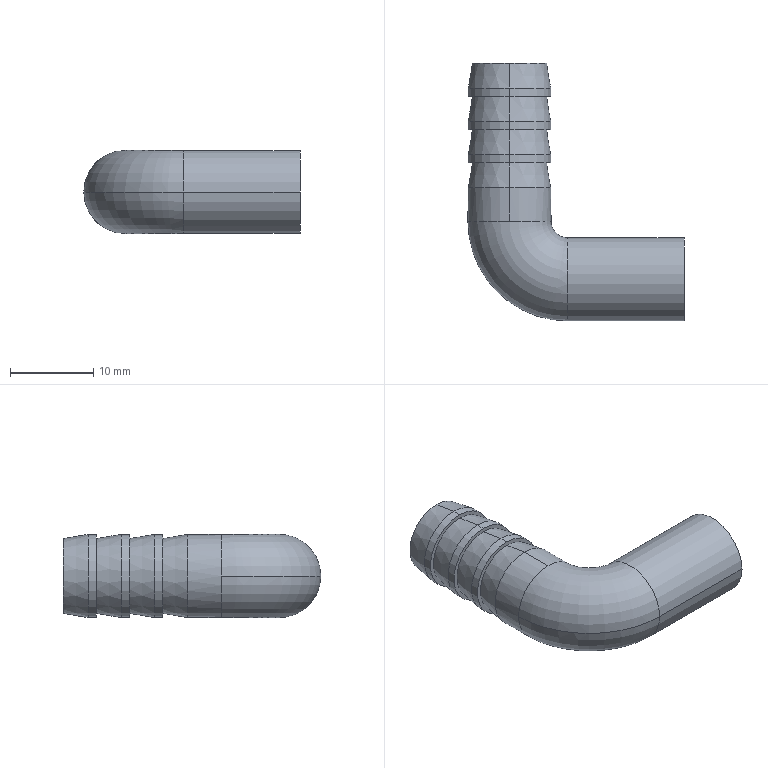Part | SolidWorks | features ICE 2, Revolution 1, Sweep 1 | 1 solid | 31 faces | box 26 x 31 x 10 mm | volume 2120 mm3 | cylinder 14 | cone 8 | plane 5 | torus 4 | commonest cylinder face diameters 10 x10 6 x4
STEP:
#1=CARTESIAN_POINT('',(7.,-10.,0.));
#2=VERTEX_POINT('',#1);
#3=CARTESIAN_POINT('',(7.,-4.,0.));
#4=VERTEX_POINT('',#3);
#5=CARTESIAN_POINT('',(7.,-7.,0.));
#6=DIRECTION('',(-1.,0.,0.));
#7=DIRECTION('',(0.,0.,-1.));
#8=AXIS2_PLACEMENT_3D('',#5,#6,#7);
#9=CIRCLE('',#8,3.);
#10=EDGE_CURVE('',#2,#4,#9,.T.);
#11=ORIENTED_EDGE('',*,*,#10,.F.);
#12=CARTESIAN_POINT('',(-3.,0.,0.));
#13=VERTEX_POINT('',#12);
#14=CARTESIAN_POINT('',(7.,0.,0.));
#15=DIRECTION('',(0.,0.,-1.));
#16=DIRECTION('',(-1.,0.,0.));
#17=AXIS2_PLACEMENT_3D('',#14,#15,#16);
#18=CIRCLE('',#17,10.);
#19=EDGE_CURVE('',#2,#13,#18,.T.);
#20=ORIENTED_EDGE('',*,*,#19,.T.);
#21=CARTESIAN_POINT('',(3.,0.,0.));
#22=VERTEX_POINT('',#21);
#23=CARTESIAN_POINT('',(0.,0.,0.));
#24=DIRECTION('',(0.,1.,0.));
#25=DIRECTION('',(0.,0.,-1.));
#26=AXIS2_PLACEMENT_3D('',#23,#24,#25);
#27=CIRCLE('',#26,3.);
#28=EDGE_CURVE('',#13,#22,#27,.T.);
#29=ORIENTED_EDGE('',*,*,#28,.T.);
#30=CARTESIAN_POINT('',(7.,0.,0.));
#31=DIRECTION('',(0.,0.,-1.));
#32=DIRECTION('',(-1.,0.,0.));
#33=AXIS2_PLACEMENT_3D('',#30,#31,#32);
#34=CIRCLE('',#33,4.);
#35=EDGE_CURVE('',#4,#22,#34,.T.);
#36=ORIENTED_EDGE('',*,*,#35,.F.);
#37=EDGE_LOOP('',(#11,#20,#29,#36));
#38=FACE_OUTER_BOUND('',#37,.T.);
#39=CARTESIAN_POINT('',(7.,0.,0.));
#40=DIRECTION('',(0.,0.,-1.));
#41=DIRECTION('',(-1.,0.,0.));
#42=AXIS2_PLACEMENT_3D('',#39,#40,#41);
#43=TOROIDAL_SURFACE('',#42,7.,3.);
#44=ADVANCED_FACE('',(#38),#43,.F.);
#45=CARTESIAN_POINT('',(7.,-12.,0.));
#46=VERTEX_POINT('',#45);
#47=CARTESIAN_POINT('',(7.,-2.,0.));
#48=VERTEX_POINT('',#47);
#49=CARTESIAN_POINT('',(7.,-7.,0.));
#50=DIRECTION('',(1.,0.,0.));
#51=DIRECTION('',(0.,0.,-1.));
#52=AXIS2_PLACEMENT_3D('',#49,#50,#51);
#53=CIRCLE('',#52,5.);
#54=EDGE_CURVE('',#46,#48,#53,.T.);
#55=ORIENTED_EDGE('',*,*,#54,.F.);
#56=CARTESIAN_POINT('',(-5.,0.,0.));
#57=VERTEX_POINT('',#56);
#58=CARTESIAN_POINT('',(7.,0.,0.));
#59=DIRECTION('',(0.,0.,-1.));
#60=DIRECTION('',(-1.,0.,0.));
#61=AXIS2_PLACEMENT_3D('',#58,#59,#60);
#62=CIRCLE('',#61,12.);
#63=EDGE_CURVE('',#46,#57,#62,.T.);
#64=ORIENTED_EDGE('',*,*,#63,.T.);
#65=CARTESIAN_POINT('',(0.,0.,-5.));
#66=VERTEX_POINT('',#65);
#67=CARTESIAN_POINT('',(0.,0.,0.));
#68=DIRECTION('',(0.,-1.,0.));
#69=DIRECTION('',(0.,0.,-1.));
#70=AXIS2_PLACEMENT_3D('',#67,#68,#69);
#71=CIRCLE('',#70,5.);
#72=EDGE_CURVE('',#57,#66,#71,.T.);
#73=ORIENTED_EDGE('',*,*,#72,.T.);
#74=CARTESIAN_POINT('',(5.,0.,0.));
#75=VERTEX_POINT('',#74);
#76=CARTESIAN_POINT('',(0.,0.,0.));
#77=DIRECTION('',(0.,-1.,0.));
#78=DIRECTION('',(0.,0.,-1.));
#79=AXIS2_PLACEMENT_3D('',#76,#77,#78);
#80=CIRCLE('',#79,5.);
#81=EDGE_CURVE('',#66,#75,#80,.T.);
#82=ORIENTED_EDGE('',*,*,#81,.T.);
#83=CARTESIAN_POINT('',(7.,0.,0.));
#84=DIRECTION('',(0.,0.,-1.));
#85=DIRECTION('',(-1.,0.,0.));
#86=AXIS2_PLACEMENT_3D('',#83,#84,#85);
#87=CIRCLE('',#86,2.);
#88=EDGE_CURVE('',#48,#75,#87,.T.);
#89=ORIENTED_EDGE('',*,*,#88,.F.);
#90=EDGE_LOOP('',(#55,#64,#73,#82,#89));
#91=FACE_OUTER_BOUND('',#90,.T.);
#92=CARTESIAN_POINT('',(7.,0.,0.));
#93=DIRECTION('',(0.,0.,-1.));
#94=DIRECTION('',(-1.,0.,0.));
#95=AXIS2_PLACEMENT_3D('',#92,#93,#94);
#96=TOROIDAL_SURFACE('',#95,7.,5.);
#97=ADVANCED_FACE('',(#91),#96,.T.);
#98=CARTESIAN_POINT('',(21.,-4.,0.));
#99=VERTEX_POINT('',#98);
#100=CARTESIAN_POINT('',(21.,-10.,0.));
#101=VERTEX_POINT('',#100);
#102=CARTESIAN_POINT('',(21.,-7.,0.));
#103=DIRECTION('',(-1.,0.,0.));
#104=DIRECTION('',(0.,0.,-1.));
#105=AXIS2_PLACEMENT_3D('',#102,#103,#104);
#106=CIRCLE('',#105,3.);
#107=EDGE_CURVE('',#99,#101,#106,.T.);
#108=ORIENTED_EDGE('',*,*,#107,.F.);
#109=CARTESIAN_POINT('',(21.,-4.,0.));
#110=DIRECTION('',(-1.,0.,0.));
#111=VECTOR('',#110,1000.);
#112=LINE('',#109,#111);
#113=EDGE_CURVE('',#99,#4,#112,.T.);
#114=ORIENTED_EDGE('',*,*,#113,.T.);
#115=CARTESIAN_POINT('',(7.,-7.,0.));
#116=DIRECTION('',(-1.,0.,0.));
#117=DIRECTION('',(0.,0.,-1.));
#118=AXIS2_PLACEMENT_3D('',#115,#116,#117);
#119=CIRCLE('',#118,3.);
#120=EDGE_CURVE('',#4,#2,#119,.T.);
#121=ORIENTED_EDGE('',*,*,#120,.T.);
#122=CARTESIAN_POINT('',(21.,-10.,0.));
#123=DIRECTION('',(-1.,0.,0.));
#124=VECTOR('',#123,1000.);
#125=LINE('',#122,#124);
#126=EDGE_CURVE('',#101,#2,#125,.T.);
#127=ORIENTED_EDGE('',*,*,#126,.F.);
#128=EDGE_LOOP('',(#108,#114,#121,#127));
#129=FACE_OUTER_BOUND('',#128,.T.);
#130=CARTESIAN_POINT('',(21.,-7.,0.));
#131=DIRECTION('',(-1.,0.,0.));
#132=DIRECTION('',(0.,-1.,0.));
#133=AXIS2_PLACEMENT_3D('',#130,#131,#132);
#134=CYLINDRICAL_SURFACE('',#133,3.);
#135=ADVANCED_FACE('',(#129),#134,.F.);
#136=CARTESIAN_POINT('',(21.,-2.,0.));
#137=VERTEX_POINT('',#136);
#138=CARTESIAN_POINT('',(21.,-12.,0.));
#139=VERTEX_POINT('',#138);
#140=CARTESIAN_POINT('',(21.,-7.,0.));
#141=DIRECTION('',(1.,0.,0.));
#142=DIRECTION('',(0.,0.,-1.));
#143=AXIS2_PLACEMENT_3D('',#140,#141,#142);
#144=CIRCLE('',#143,5.);
#145=EDGE_CURVE('',#137,#139,#144,.T.);
#146=ORIENTED_EDGE('',*,*,#145,.F.);
#147=CARTESIAN_POINT('',(21.,-2.,0.));
#148=DIRECTION('',(-1.,0.,0.));
#149=VECTOR('',#148,1000.);
#150=LINE('',#147,#149);
#151=EDGE_CURVE('',#137,#48,#150,.T.);
#152=ORIENTED_EDGE('',*,*,#151,.T.);
#153=CARTESIAN_POINT('',(7.,-7.,0.));
#154=DIRECTION('',(1.,0.,0.));
#155=DIRECTION('',(0.,0.,-1.));
#156=AXIS2_PLACEMENT_3D('',#153,#154,#155);
#157=CIRCLE('',#156,5.);
#158=EDGE_CURVE('',#48,#46,#157,.T.);
#159=ORIENTED_EDGE('',*,*,#158,.T.);
#160=CARTESIAN_POINT('',(21.,-12.,0.));
#161=DIRECTION('',(-1.,0.,0.));
#162=VECTOR('',#161,1000.);
#163=LINE('',#160,#162);
#164=EDGE_CURVE('',#139,#46,#163,.T.);
#165=ORIENTED_EDGE('',*,*,#164,.F.);
#166=EDGE_LOOP('',(#146,#152,#159,#165));
#167=FACE_OUTER_BOUND('',#166,.T.);
#168=CARTESIAN_POINT('',(21.,-7.,0.));
#169=DIRECTION('',(-1.,0.,0.));
#170=DIRECTION('',(0.,-1.,0.));
#171=AXIS2_PLACEMENT_3D('',#168,#169,#170);
#172=CYLINDRICAL_SURFACE('',#171,5.);
#173=ADVANCED_FACE('',(#167),#172,.T.);
#174=CARTESIAN_POINT('',(0.,0.,0.));
#175=DIRECTION('',(0.,1.,0.));
#176=DIRECTION('',(0.,0.,-1.));
#177=AXIS2_PLACEMENT_3D('',#174,#175,#176);
#178=CIRCLE('',#177,3.);
#179=EDGE_CURVE('',#22,#13,#178,.T.);
#180=ORIENTED_EDGE('',*,*,#179,.F.);
#181=CARTESIAN_POINT('',(3.,19.,0.));
#182=VERTEX_POINT('',#181);
#183=CARTESIAN_POINT('',(3.,-0.001,0.));
#184=DIRECTION('',(0.,1.,0.));
#185=VECTOR('',#184,1000.);
#186=LINE('',#183,#185);
#187=EDGE_CURVE('',#22,#182,#186,.T.);
#188=ORIENTED_EDGE('',*,*,#187,.T.);
#189=CARTESIAN_POINT('',(-3.,19.,0.));
#190=VERTEX_POINT('',#189);
#191=CARTESIAN_POINT('',(0.,19.,0.));
#192=DIRECTION('',(0.,1.,0.));
#193=DIRECTION('',(-1.,0.,0.));
#194=AXIS2_PLACEMENT_3D('',#191,#192,#193);
#195=CIRCLE('',#194,3.);
#196=EDGE_CURVE('',#182,#190,#195,.T.);
#197=ORIENTED_EDGE('',*,*,#196,.T.);
#198=CARTESIAN_POINT('',(-3.,-0.001,0.));
#199=DIRECTION('',(0.,1.,0.));
#200=VECTOR('',#199,1000.);
#201=LINE('',#198,#200);
#202=EDGE_CURVE('',#13,#190,#201,.T.);
#203=ORIENTED_EDGE('',*,*,#202,.F.);
#204=EDGE_LOOP('',(#180,#188,#197,#203));
#205=FACE_OUTER_BOUND('',#204,.T.);
#206=CARTESIAN_POINT('',(0.,-0.001,0.));
#207=DIRECTION('',(0.,1.,0.));
#208=DIRECTION('',(-1.,0.,0.));
#209=AXIS2_PLACEMENT_3D('',#206,#207,#208);
#210=CYLINDRICAL_SURFACE('',#209,3.);
#211=ADVANCED_FACE('',(#205),#210,.F.);
#212=CARTESIAN_POINT('',(0.,19.,-4.5));
#213=VERTEX_POINT('',#212);
#214=CARTESIAN_POINT('',(0.,19.,4.5));
#215=VERTEX_POINT('',#214);
#216=CARTESIAN_POINT('',(0.,19.,0.));
#217=DIRECTION('',(0.,-1.,0.));
#218=DIRECTION('',(0.,0.,-1.));
#219=AXIS2_PLACEMENT_3D('',#216,#217,#218);
#220=CIRCLE('',#219,4.5);
#221=EDGE_CURVE('',#213,#215,#220,.T.);
#222=ORIENTED_EDGE('',*,*,#221,.T.);
#223=CARTESIAN_POINT('',(0.,16.,5.));
#224=VERTEX_POINT('',#223);
#225=CARTESIAN_POINT('',(0.,19.,4.5));
#226=DIRECTION('',(0.,-0.9864,0.1644));
#227=VECTOR('',#226,1000.);
#228=LINE('',#225,#227);
#229=EDGE_CURVE('',#215,#224,#228,.T.);
#230=ORIENTED_EDGE('',*,*,#229,.T.);
#231=CARTESIAN_POINT('',(0.,16.,-5.));
#232=VERTEX_POINT('',#231);
#233=CARTESIAN_POINT('',(0.,16.,0.));
#234=DIRECTION('',(0.,-1.,0.));
#235=DIRECTION('',(0.,0.,-1.));
#236=AXIS2_PLACEMENT_3D('',#233,#234,#235);
#237=CIRCLE('',#236,5.);
#238=EDGE_CURVE('',#232,#224,#237,.T.);
#239=ORIENTED_EDGE('',*,*,#238,.F.);
#240=CARTESIAN_POINT('',(0.,19.,-4.5));
#241=DIRECTION('',(0.,-0.9864,-0.1644));
#242=VECTOR('',#241,1000.);
#243=LINE('',#240,#242);
#244=EDGE_CURVE('',#213,#232,#243,.T.);
#245=ORIENTED_EDGE('',*,*,#244,.F.);
#246=EDGE_LOOP('',(#222,#230,#239,#245));
#247=FACE_OUTER_BOUND('',#246,.T.);
#248=CARTESIAN_POINT('',(0.,19.,0.));
#249=DIRECTION('',(0.,-1.,0.));
#250=DIRECTION('',(0.,0.,-1.));
#251=AXIS2_PLACEMENT_3D('',#248,#249,#250);
#252=CONICAL_SURFACE('',#251,4.5,0.1651);
#253=ADVANCED_FACE('',(#247),#252,.T.);
#254=ORIENTED_EDGE('',*,*,#238,.T.);
#255=CARTESIAN_POINT('',(0.,15.,5.));
#256=VERTEX_POINT('',#255);
#257=CARTESIAN_POINT('',(0.,0.,5.));
#258=DIRECTION('',(0.,-1.,0.));
#259=VECTOR('',#258,1000.);
#260=LINE('',#257,#259);
#261=EDGE_CURVE('',#224,#256,#260,.T.);
#262=ORIENTED_EDGE('',*,*,#261,.T.);
#263=CARTESIAN_POINT('',(0.,15.,-5.));
#264=VERTEX_POINT('',#263);
#265=CARTESIAN_POINT('',(0.,15.,0.));
#266=DIRECTION('',(0.,-1.,0.));
#267=DIRECTION('',(0.,0.,-1.));
#268=AXIS2_PLACEMENT_3D('',#265,#266,#267);
#269=CIRCLE('',#268,5.);
#270=EDGE_CURVE('',#264,#256,#269,.T.);
#271=ORIENTED_EDGE('',*,*,#270,.F.);
#272=CARTESIAN_POINT('',(0.,0.,-5.));
#273=DIRECTION('',(0.,-1.,0.));
#274=VECTOR('',#273,1000.);
#275=LINE('',#272,#274);
#276=EDGE_CURVE('',#232,#264,#275,.T.);
#277=ORIENTED_EDGE('',*,*,#276,.F.);
#278=EDGE_LOOP('',(#254,#262,#271,#277));
#279=FACE_OUTER_BOUND('',#278,.T.);
#280=CARTESIAN_POINT('',(0.,0.,0.));
#281=DIRECTION('',(0.,-1.,0.));
#282=DIRECTION('',(0.,0.,-1.));
#283=AXIS2_PLACEMENT_3D('',#280,#281,#282);
#284=CYLINDRICAL_SURFACE('',#283,5.);
#285=ADVANCED_FACE('',(#279),#284,.T.);
#286=CARTESIAN_POINT('',(0.,15.,-4.5));
#287=VERTEX_POINT('',#286);
#288=CARTESIAN_POINT('',(0.,15.,4.5));
#289=VERTEX_POINT('',#288);
#290=CARTESIAN_POINT('',(0.,15.,0.));
#291=DIRECTION('',(0.,-1.,0.));
#292=DIRECTION('',(0.,0.,-1.));
#293=AXIS2_PLACEMENT_3D('',#290,#291,#292);
#294=CIRCLE('',#293,4.5);
#295=EDGE_CURVE('',#287,#289,#294,.T.);
#296=ORIENTED_EDGE('',*,*,#295,.T.);
#297=CARTESIAN_POINT('',(0.,12.,5.));
#298=VERTEX_POINT('',#297);
#299=CARTESIAN_POINT('',(0.,15.,4.5));
#300=DIRECTION('',(0.,-0.9864,0.1644));
#301=VECTOR('',#300,1000.);
#302=LINE('',#299,#301);
#303=EDGE_CURVE('',#289,#298,#302,.T.);
#304=ORIENTED_EDGE('',*,*,#303,.T.);
#305=CARTESIAN_POINT('',(0.,12.,-5.));
#306=VERTEX_POINT('',#305);
#307=CARTESIAN_POINT('',(0.,12.,0.));
#308=DIRECTION('',(0.,-1.,0.));
#309=DIRECTION('',(0.,0.,-1.));
#310=AXIS2_PLACEMENT_3D('',#307,#308,#309);
#311=CIRCLE('',#310,5.);
#312=EDGE_CURVE('',#306,#298,#311,.T.);
#313=ORIENTED_EDGE('',*,*,#312,.F.);
#314=CARTESIAN_POINT('',(0.,15.,-4.5));
#315=DIRECTION('',(0.,-0.9864,-0.1644));
#316=VECTOR('',#315,1000.);
#317=LINE('',#314,#316);
#318=EDGE_CURVE('',#287,#306,#317,.T.);
#319=ORIENTED_EDGE('',*,*,#318,.F.);
#320=EDGE_LOOP('',(#296,#304,#313,#319));
#321=FACE_OUTER_BOUND('',#320,.T.);
#322=CARTESIAN_POINT('',(0.,15.,0.));
#323=DIRECTION('',(0.,-1.,0.));
#324=DIRECTION('',(0.,0.,-1.));
#325=AXIS2_PLACEMENT_3D('',#322,#323,#324);
#326=CONICAL_SURFACE('',#325,4.5,0.1651);
#327=ADVANCED_FACE('',(#321),#326,.T.);
#328=ORIENTED_EDGE('',*,*,#312,.T.);
#329=CARTESIAN_POINT('',(0.,11.,5.));
#330=VERTEX_POINT('',#329);
#331=CARTESIAN_POINT('',(0.,0.,5.));
#332=DIRECTION('',(0.,-1.,0.));
#333=VECTOR('',#332,1000.);
#334=LINE('',#331,#333);
#335=EDGE_CURVE('',#298,#330,#334,.T.);
#336=ORIENTED_EDGE('',*,*,#335,.T.);
#337=CARTESIAN_POINT('',(0.,11.,-5.));
#338=VERTEX_POINT('',#337);
#339=CARTESIAN_POINT('',(0.,11.,0.));
#340=DIRECTION('',(0.,-1.,0.));
#341=DIRECTION('',(0.,0.,-1.));
#342=AXIS2_PLACEMENT_3D('',#339,#340,#341);
#343=CIRCLE('',#342,5.);
#344=EDGE_CURVE('',#338,#330,#343,.T.);
#345=ORIENTED_EDGE('',*,*,#344,.F.);
#346=CARTESIAN_POINT('',(0.,0.,-5.));
#347=DIRECTION('',(0.,-1.,0.));
#348=VECTOR('',#347,1000.);
#349=LINE('',#346,#348);
#350=EDGE_CURVE('',#306,#338,#349,.T.);
#351=ORIENTED_EDGE('',*,*,#350,.F.);
#352=EDGE_LOOP('',(#328,#336,#345,#351));
#353=FACE_OUTER_BOUND('',#352,.T.);
#354=CARTESIAN_POINT('',(0.,0.,0.));
#355=DIRECTION('',(0.,-1.,0.));
#356=DIRECTION('',(0.,0.,-1.));
#357=AXIS2_PLACEMENT_3D('',#354,#355,#356);
#358=CYLINDRICAL_SURFACE('',#357,5.);
#359=ADVANCED_FACE('',(#353),#358,.T.);
#360=CARTESIAN_POINT('',(0.,11.,-4.5));
#361=VERTEX_POINT('',#360);
#362=CARTESIAN_POINT('',(0.,11.,4.5));
#363=VERTEX_POINT('',#362);
#364=CARTESIAN_POINT('',(0.,11.,0.));
#365=DIRECTION('',(0.,-1.,0.));
#366=DIRECTION('',(0.,0.,-1.));
#367=AXIS2_PLACEMENT_3D('',#364,#365,#366);
#368=CIRCLE('',#367,4.5);
#369=EDGE_CURVE('',#361,#363,#368,.T.);
#370=ORIENTED_EDGE('',*,*,#369,.T.);
#371=CARTESIAN_POINT('',(0.,8.,5.));
#372=VERTEX_POINT('',#371);
#373=CARTESIAN_POINT('',(0.,11.,4.5));
#374=DIRECTION('',(0.,-0.9864,0.1644));
#375=VECTOR('',#374,1000.);
#376=LINE('',#373,#375);
#377=EDGE_CURVE('',#363,#372,#376,.T.);
#378=ORIENTED_EDGE('',*,*,#377,.T.);
#379=CARTESIAN_POINT('',(0.,8.,-5.));
#380=VERTEX_POINT('',#379);
#381=CARTESIAN_POINT('',(0.,8.,0.));
#382=DIRECTION('',(0.,-1.,0.));
#383=DIRECTION('',(0.,0.,-1.));
#384=AXIS2_PLACEMENT_3D('',#381,#382,#383);
#385=CIRCLE('',#384,5.);
#386=EDGE_CURVE('',#380,#372,#385,.T.);
#387=ORIENTED_EDGE('',*,*,#386,.F.);
#388=CARTESIAN_POINT('',(0.,11.,-4.5));
#389=DIRECTION('',(0.,-0.9864,-0.1644));
#390=VECTOR('',#389,1000.);
#391=LINE('',#388,#390);
#392=EDGE_CURVE('',#361,#380,#391,.T.);
#393=ORIENTED_EDGE('',*,*,#392,.F.);
#394=EDGE_LOOP('',(#370,#378,#387,#393));
#395=FACE_OUTER_BOUND('',#394,.T.);
#396=CARTESIAN_POINT('',(0.,11.,0.));
#397=DIRECTION('',(0.,-1.,0.));
#398=DIRECTION('',(0.,0.,-1.));
#399=AXIS2_PLACEMENT_3D('',#396,#397,#398);
#400=CONICAL_SURFACE('',#399,4.5,0.1651);
#401=ADVANCED_FACE('',(#395),#400,.T.);
#402=ORIENTED_EDGE('',*,*,#386,.T.);
#403=CARTESIAN_POINT('',(0.,7.,5.));
#404=VERTEX_POINT('',#403);
#405=CARTESIAN_POINT('',(0.,0.,5.));
#406=DIRECTION('',(0.,-1.,0.));
#407=VECTOR('',#406,1000.);
#408=LINE('',#405,#407);
#409=EDGE_CURVE('',#372,#404,#408,.T.);
#410=ORIENTED_EDGE('',*,*,#409,.T.);
#411=CARTESIAN_POINT('',(0.,7.,-5.));
#412=VERTEX_POINT('',#411);
#413=CARTESIAN_POINT('',(0.,7.,0.));
#414=DIRECTION('',(0.,-1.,0.));
#415=DIRECTION('',(0.,0.,-1.));
#416=AXIS2_PLACEMENT_3D('',#413,#414,#415);
#417=CIRCLE('',#416,5.);
#418=EDGE_CURVE('',#412,#404,#417,.T.);
#419=ORIENTED_EDGE('',*,*,#418,.F.);
#420=CARTESIAN_POINT('',(0.,0.,-5.));
#421=DIRECTION('',(0.,-1.,0.));
#422=VECTOR('',#421,1000.);
#423=LINE('',#420,#422);
#424=EDGE_CURVE('',#380,#412,#423,.T.);
#425=ORIENTED_EDGE('',*,*,#424,.F.);
#426=EDGE_LOOP('',(#402,#410,#419,#425));
#427=FACE_OUTER_BOUND('',#426,.T.);
#428=CARTESIAN_POINT('',(0.,0.,0.));
#429=DIRECTION('',(0.,-1.,0.));
#430=DIRECTION('',(0.,0.,-1.));
#431=AXIS2_PLACEMENT_3D('',#428,#429,#430);
#432=CYLINDRICAL_SURFACE('',#431,5.);
#433=ADVANCED_FACE('',(#427),#432,.T.);
#434=CARTESIAN_POINT('',(0.,7.,-4.5));
#435=VERTEX_POINT('',#434);
#436=CARTESIAN_POINT('',(0.,7.,4.5));
#437=VERTEX_POINT('',#436);
#438=CARTESIAN_POINT('',(0.,7.,0.));
#439=DIRECTION('',(0.,-1.,0.));
#440=DIRECTION('',(0.,0.,-1.));
#441=AXIS2_PLACEMENT_3D('',#438,#439,#440);
#442=CIRCLE('',#441,4.5);
#443=EDGE_CURVE('',#435,#437,#442,.T.);
#444=ORIENTED_EDGE('',*,*,#443,.T.);
#445=CARTESIAN_POINT('',(0.,4.,5.));
#446=VERTEX_POINT('',#445);
#447=CARTESIAN_POINT('',(0.,7.,4.5));
#448=DIRECTION('',(0.,-0.9864,0.1644));
#449=VECTOR('',#448,1000.);
#450=LINE('',#447,#449);
#451=EDGE_CURVE('',#437,#446,#450,.T.);
#452=ORIENTED_EDGE('',*,*,#451,.T.);
#453=CARTESIAN_POINT('',(0.,4.,-5.));
#454=VERTEX_POINT('',#453);
#455=CARTESIAN_POINT('',(0.,4.,0.));
#456=DIRECTION('',(0.,-1.,0.));
#457=DIRECTION('',(0.,0.,-1.));
#458=AXIS2_PLACEMENT_3D('',#455,#456,#457);
#459=CIRCLE('',#458,5.);
#460=EDGE_CURVE('',#454,#446,#459,.T.);
#461=ORIENTED_EDGE('',*,*,#460,.F.);
#462=CARTESIAN_POINT('',(0.,7.,-4.5));
#463=DIRECTION('',(0.,-0.9864,-0.1644));
#464=VECTOR('',#463,1000.);
#465=LINE('',#462,#464);
#466=EDGE_CURVE('',#435,#454,#465,.T.);
#467=ORIENTED_EDGE('',*,*,#466,.F.);
#468=EDGE_LOOP('',(#444,#452,#461,#467));
#469=FACE_OUTER_BOUND('',#468,.T.);
#470=CARTESIAN_POINT('',(0.,7.,0.));
#471=DIRECTION('',(0.,-1.,0.));
#472=DIRECTION('',(0.,0.,-1.));
#473=AXIS2_PLACEMENT_3D('',#470,#471,#472);
#474=CONICAL_SURFACE('',#473,4.5,0.1651);
#475=ADVANCED_FACE('',(#469),#474,.T.);
#476=ORIENTED_EDGE('',*,*,#460,.T.);
#477=CARTESIAN_POINT('',(0.,0.,5.));
#478=VERTEX_POINT('',#477);
#479=CARTESIAN_POINT('',(0.,0.,5.));
#480=DIRECTION('',(0.,-1.,0.));
#481=VECTOR('',#480,1000.);
#482=LINE('',#479,#481);
#483=EDGE_CURVE('',#446,#478,#482,.T.);
#484=ORIENTED_EDGE('',*,*,#483,.T.);
#485=CARTESIAN_POINT('',(0.,0.,0.));
#486=DIRECTION('',(0.,-1.,0.));
#487=DIRECTION('',(0.,0.,-1.));
#488=AXIS2_PLACEMENT_3D('',#485,#486,#487);
#489=CIRCLE('',#488,5.);
#490=EDGE_CURVE('',#75,#478,#489,.T.);
#491=ORIENTED_EDGE('',*,*,#490,.F.);
#492=ORIENTED_EDGE('',*,*,#81,.F.);
#493=CARTESIAN_POINT('',(0.,0.,-5.));
#494=DIRECTION('',(0.,-1.,0.));
#495=VECTOR('',#494,1000.);
#496=LINE('',#493,#495);
#497=EDGE_CURVE('',#454,#66,#496,.T.);
#498=ORIENTED_EDGE('',*,*,#497,.F.);
#499=EDGE_LOOP('',(#476,#484,#491,#492,#498));
#500=FACE_OUTER_BOUND('',#499,.T.);
#501=CARTESIAN_POINT('',(0.,0.,0.));
#502=DIRECTION('',(0.,-1.,0.));
#503=DIRECTION('',(0.,0.,-1.));
#504=AXIS2_PLACEMENT_3D('',#501,#502,#503);
#505=CYLINDRICAL_SURFACE('',#504,5.);
#506=ADVANCED_FACE('',(#500),#505,.T.);
#507=ORIENTED_EDGE('',*,*,#483,.F.);
#508=CARTESIAN_POINT('',(0.,4.,0.));
#509=DIRECTION('',(0.,-1.,0.));
#510=DIRECTION('',(0.,0.,-1.));
#511=AXIS2_PLACEMENT_3D('',#508,#509,#510);
#512=CIRCLE('',#511,5.);
#513=EDGE_CURVE('',#446,#454,#512,.T.);
#514=ORIENTED_EDGE('',*,*,#513,.T.);
#515=ORIENTED_EDGE('',*,*,#497,.T.);
#516=ORIENTED_EDGE('',*,*,#72,.F.);
#517=CARTESIAN_POINT('',(0.,0.,0.));
#518=DIRECTION('',(0.,-1.,0.));
#519=DIRECTION('',(0.,0.,-1.));
#520=AXIS2_PLACEMENT_3D('',#517,#518,#519);
#521=CIRCLE('',#520,5.);
#522=EDGE_CURVE('',#478,#57,#521,.T.);
#523=ORIENTED_EDGE('',*,*,#522,.F.);
#524=EDGE_LOOP('',(#507,#514,#515,#516,#523));
#525=FACE_OUTER_BOUND('',#524,.T.);
#526=CARTESIAN_POINT('',(0.,0.,0.));
#527=DIRECTION('',(0.,-1.,0.));
#528=DIRECTION('',(0.,0.,-1.));
#529=AXIS2_PLACEMENT_3D('',#526,#527,#528);
#530=CYLINDRICAL_SURFACE('',#529,5.);
#531=ADVANCED_FACE('',(#525),#530,.T.);
#532=ORIENTED_EDGE('',*,*,#451,.F.);
#533=CARTESIAN_POINT('',(0.,7.,0.));
#534=DIRECTION('',(0.,-1.,0.));
#535=DIRECTION('',(0.,0.,-1.));
#536=AXIS2_PLACEMENT_3D('',#533,#534,#535);
#537=CIRCLE('',#536,4.5);
#538=EDGE_CURVE('',#437,#435,#537,.T.);
#539=ORIENTED_EDGE('',*,*,#538,.T.);
#540=ORIENTED_EDGE('',*,*,#466,.T.);
#541=ORIENTED_EDGE('',*,*,#513,.F.);
#542=EDGE_LOOP('',(#532,#539,#540,#541));
#543=FACE_OUTER_BOUND('',#542,.T.);
#544=CARTESIAN_POINT('',(0.,7.,0.));
#545=DIRECTION('',(0.,-1.,0.));
#546=DIRECTION('',(0.,0.,-1.));
#547=AXIS2_PLACEMENT_3D('',#544,#545,#546);
#548=CONICAL_SURFACE('',#547,4.5,0.1651);
#549=ADVANCED_FACE('',(#543),#548,.T.);
#550=ORIENTED_EDGE('',*,*,#443,.F.);
#551=ORIENTED_EDGE('',*,*,#538,.F.);
#552=EDGE_LOOP('',(#550,#551));
#553=FACE_BOUND('',#552,.T.);
#554=ORIENTED_EDGE('',*,*,#418,.T.);
#555=CARTESIAN_POINT('',(0.,7.,0.));
#556=DIRECTION('',(0.,-1.,0.));
#557=DIRECTION('',(0.,0.,-1.));
#558=AXIS2_PLACEMENT_3D('',#555,#556,#557);
#559=CIRCLE('',#558,5.);
#560=EDGE_CURVE('',#404,#412,#559,.T.);
#561=ORIENTED_EDGE('',*,*,#560,.T.);
#562=EDGE_LOOP('',(#554,#561));
#563=FACE_OUTER_BOUND('',#562,.T.);
#564=CARTESIAN_POINT('',(-5.,7.,0.));
#565=DIRECTION('',(0.,1.,0.));
#566=DIRECTION('',(0.,0.,1.));
#567=AXIS2_PLACEMENT_3D('',#564,#565,#566);
#568=PLANE('',#567);
#569=ADVANCED_FACE('',(#553,#563),#568,.F.);
#570=ORIENTED_EDGE('',*,*,#409,.F.);
#571=CARTESIAN_POINT('',(0.,8.,0.));
#572=DIRECTION('',(0.,-1.,0.));
#573=DIRECTION('',(0.,0.,-1.));
#574=AXIS2_PLACEMENT_3D('',#571,#572,#573);
#575=CIRCLE('',#574,5.);
#576=EDGE_CURVE('',#372,#380,#575,.T.);
#577=ORIENTED_EDGE('',*,*,#576,.T.);
#578=ORIENTED_EDGE('',*,*,#424,.T.);
#579=ORIENTED_EDGE('',*,*,#560,.F.);
#580=EDGE_LOOP('',(#570,#577,#578,#579));
#581=FACE_OUTER_BOUND('',#580,.T.);
#582=CARTESIAN_POINT('',(0.,0.,0.));
#583=DIRECTION('',(0.,-1.,0.));
#584=DIRECTION('',(0.,0.,-1.));
#585=AXIS2_PLACEMENT_3D('',#582,#583,#584);
#586=CYLINDRICAL_SURFACE('',#585,5.);
#587=ADVANCED_FACE('',(#581),#586,.T.);
#588=ORIENTED_EDGE('',*,*,#377,.F.);
#589=CARTESIAN_POINT('',(0.,11.,0.));
#590=DIRECTION('',(0.,-1.,0.));
#591=DIRECTION('',(0.,0.,-1.));
#592=AXIS2_PLACEMENT_3D('',#589,#590,#591);
#593=CIRCLE('',#592,4.5);
#594=EDGE_CURVE('',#363,#361,#593,.T.);
#595=ORIENTED_EDGE('',*,*,#594,.T.);
#596=ORIENTED_EDGE('',*,*,#392,.T.);
#597=ORIENTED_EDGE('',*,*,#576,.F.);
#598=EDGE_LOOP('',(#588,#595,#596,#597));
#599=FACE_OUTER_BOUND('',#598,.T.);
#600=CARTESIAN_POINT('',(0.,11.,0.));
#601=DIRECTION('',(0.,-1.,0.));
#602=DIRECTION('',(0.,0.,-1.));
#603=AXIS2_PLACEMENT_3D('',#600,#601,#602);
#604=CONICAL_SURFACE('',#603,4.5,0.1651);
#605=ADVANCED_FACE('',(#599),#604,.T.);
#606=ORIENTED_EDGE('',*,*,#369,.F.);
#607=ORIENTED_EDGE('',*,*,#594,.F.);
#608=EDGE_LOOP('',(#606,#607));
#609=FACE_BOUND('',#608,.T.);
#610=ORIENTED_EDGE('',*,*,#344,.T.);
#611=CARTESIAN_POINT('',(0.,11.,0.));
#612=DIRECTION('',(0.,-1.,0.));
#613=DIRECTION('',(0.,0.,-1.));
#614=AXIS2_PLACEMENT_3D('',#611,#612,#613);
#615=CIRCLE('',#614,5.);
#616=EDGE_CURVE('',#330,#338,#615,.T.);
#617=ORIENTED_EDGE('',*,*,#616,.T.);
#618=EDGE_LOOP('',(#610,#617));
#619=FACE_OUTER_BOUND('',#618,.T.);
#620=CARTESIAN_POINT('',(-5.,11.,0.));
#621=DIRECTION('',(0.,1.,0.));
#622=DIRECTION('',(0.,0.,1.));
#623=AXIS2_PLACEMENT_3D('',#620,#621,#622);
#624=PLANE('',#623);
#625=ADVANCED_FACE('',(#609,#619),#624,.F.);
#626=ORIENTED_EDGE('',*,*,#335,.F.);
#627=CARTESIAN_POINT('',(0.,12.,0.));
#628=DIRECTION('',(0.,-1.,0.));
#629=DIRECTION('',(0.,0.,-1.));
#630=AXIS2_PLACEMENT_3D('',#627,#628,#629);
#631=CIRCLE('',#630,5.);
#632=EDGE_CURVE('',#298,#306,#631,.T.);
#633=ORIENTED_EDGE('',*,*,#632,.T.);
#634=ORIENTED_EDGE('',*,*,#350,.T.);
#635=ORIENTED_EDGE('',*,*,#616,.F.);
#636=EDGE_LOOP('',(#626,#633,#634,#635));
#637=FACE_OUTER_BOUND('',#636,.T.);
#638=CARTESIAN_POINT('',(0.,0.,0.));
#639=DIRECTION('',(0.,-1.,0.));
#640=DIRECTION('',(0.,0.,-1.));
#641=AXIS2_PLACEMENT_3D('',#638,#639,#640);
#642=CYLINDRICAL_SURFACE('',#641,5.);
#643=ADVANCED_FACE('',(#637),#642,.T.);
#644=ORIENTED_EDGE('',*,*,#303,.F.);
#645=CARTESIAN_POINT('',(0.,15.,0.));
#646=DIRECTION('',(0.,-1.,0.));
#647=DIRECTION('',(0.,0.,-1.));
#648=AXIS2_PLACEMENT_3D('',#645,#646,#647);
#649=CIRCLE('',#648,4.5);
#650=EDGE_CURVE('',#289,#287,#649,.T.);
#651=ORIENTED_EDGE('',*,*,#650,.T.);
#652=ORIENTED_EDGE('',*,*,#318,.T.);
#653=ORIENTED_EDGE('',*,*,#632,.F.);
#654=EDGE_LOOP('',(#644,#651,#652,#653));
#655=FACE_OUTER_BOUND('',#654,.T.);
#656=CARTESIAN_POINT('',(0.,15.,0.));
#657=DIRECTION('',(0.,-1.,0.));
#658=DIRECTION('',(0.,0.,-1.));
#659=AXIS2_PLACEMENT_3D('',#656,#657,#658);
#660=CONICAL_SURFACE('',#659,4.5,0.1651);
#661=ADVANCED_FACE('',(#655),#660,.T.);
#662=ORIENTED_EDGE('',*,*,#295,.F.);
#663=ORIENTED_EDGE('',*,*,#650,.F.);
#664=EDGE_LOOP('',(#662,#663));
#665=FACE_BOUND('',#664,.T.);
#666=ORIENTED_EDGE('',*,*,#270,.T.);
#667=CARTESIAN_POINT('',(0.,15.,0.));
#668=DIRECTION('',(0.,-1.,0.));
#669=DIRECTION('',(0.,0.,-1.));
#670=AXIS2_PLACEMENT_3D('',#667,#668,#669);
#671=CIRCLE('',#670,5.);
#672=EDGE_CURVE('',#256,#264,#671,.T.);
#673=ORIENTED_EDGE('',*,*,#672,.T.);
#674=EDGE_LOOP('',(#666,#673));
#675=FACE_OUTER_BOUND('',#674,.T.);
#676=CARTESIAN_POINT('',(-5.,15.,0.));
#677=DIRECTION('',(0.,1.,0.));
#678=DIRECTION('',(0.,0.,1.));
#679=AXIS2_PLACEMENT_3D('',#676,#677,#678);
#680=PLANE('',#679);
#681=ADVANCED_FACE('',(#665,#675),#680,.F.);
#682=ORIENTED_EDGE('',*,*,#261,.F.);
#683=CARTESIAN_POINT('',(0.,16.,0.));
#684=DIRECTION('',(0.,-1.,0.));
#685=DIRECTION('',(0.,0.,-1.));
#686=AXIS2_PLACEMENT_3D('',#683,#684,#685);
#687=CIRCLE('',#686,5.);
#688=EDGE_CURVE('',#224,#232,#687,.T.);
#689=ORIENTED_EDGE('',*,*,#688,.T.);
#690=ORIENTED_EDGE('',*,*,#276,.T.);
#691=ORIENTED_EDGE('',*,*,#672,.F.);
#692=EDGE_LOOP('',(#682,#689,#690,#691));
#693=FACE_OUTER_BOUND('',#692,.T.);
#694=CARTESIAN_POINT('',(0.,0.,0.));
#695=DIRECTION('',(0.,-1.,0.));
#696=DIRECTION('',(0.,0.,-1.));
#697=AXIS2_PLACEMENT_3D('',#694,#695,#696);
#698=CYLINDRICAL_SURFACE('',#697,5.);
#699=ADVANCED_FACE('',(#693),#698,.T.);
#700=ORIENTED_EDGE('',*,*,#229,.F.);
#701=CARTESIAN_POINT('',(0.,19.,0.));
#702=DIRECTION('',(0.,-1.,0.));
#703=DIRECTION('',(0.,0.,-1.));
#704=AXIS2_PLACEMENT_3D('',#701,#702,#703);
#705=CIRCLE('',#704,4.5);
#706=EDGE_CURVE('',#215,#213,#705,.T.);
#707=ORIENTED_EDGE('',*,*,#706,.T.);
#708=ORIENTED_EDGE('',*,*,#244,.T.);
#709=ORIENTED_EDGE('',*,*,#688,.F.);
#710=EDGE_LOOP('',(#700,#707,#708,#709));
#711=FACE_OUTER_BOUND('',#710,.T.);
#712=CARTESIAN_POINT('',(0.,19.,0.));
#713=DIRECTION('',(0.,-1.,0.));
#714=DIRECTION('',(0.,0.,-1.));
#715=AXIS2_PLACEMENT_3D('',#712,#713,#714);
#716=CONICAL_SURFACE('',#715,4.5,0.1651);
#717=ADVANCED_FACE('',(#711),#716,.T.);
#718=CARTESIAN_POINT('',(0.,19.,0.));
#719=DIRECTION('',(0.,1.,0.));
#720=DIRECTION('',(-1.,0.,0.));
#721=AXIS2_PLACEMENT_3D('',#718,#719,#720);
#722=CIRCLE('',#721,3.);
#723=EDGE_CURVE('',#190,#182,#722,.T.);
#724=ORIENTED_EDGE('',*,*,#723,.F.);
#725=ORIENTED_EDGE('',*,*,#196,.F.);
#726=EDGE_LOOP('',(#724,#725));
#727=FACE_BOUND('',#726,.T.);
#728=ORIENTED_EDGE('',*,*,#221,.F.);
#729=ORIENTED_EDGE('',*,*,#706,.F.);
#730=EDGE_LOOP('',(#728,#729));
#731=FACE_OUTER_BOUND('',#730,.T.);
#732=CARTESIAN_POINT('',(-4.5,19.,0.));
#733=DIRECTION('',(0.,-1.,0.));
#734=DIRECTION('',(0.,0.,-1.));
#735=AXIS2_PLACEMENT_3D('',#732,#733,#734);
#736=PLANE('',#735);
#737=ADVANCED_FACE('',(#727,#731),#736,.F.);
#738=ORIENTED_EDGE('',*,*,#187,.F.);
#739=ORIENTED_EDGE('',*,*,#28,.F.);
#740=ORIENTED_EDGE('',*,*,#202,.T.);
#741=ORIENTED_EDGE('',*,*,#723,.T.);
#742=EDGE_LOOP('',(#738,#739,#740,#741));
#743=FACE_OUTER_BOUND('',#742,.T.);
#744=CARTESIAN_POINT('',(0.,-0.001,0.));
#745=DIRECTION('',(0.,1.,0.));
#746=DIRECTION('',(-1.,0.,0.));
#747=AXIS2_PLACEMENT_3D('',#744,#745,#746);
#748=CYLINDRICAL_SURFACE('',#747,3.);
#749=ADVANCED_FACE('',(#743),#748,.F.);
#750=ORIENTED_EDGE('',*,*,#19,.F.);
#751=ORIENTED_EDGE('',*,*,#120,.F.);
#752=ORIENTED_EDGE('',*,*,#35,.T.);
#753=ORIENTED_EDGE('',*,*,#179,.T.);
#754=EDGE_LOOP('',(#750,#751,#752,#753));
#755=FACE_OUTER_BOUND('',#754,.T.);
#756=CARTESIAN_POINT('',(7.,0.,0.));
#757=DIRECTION('',(0.,0.,-1.));
#758=DIRECTION('',(-1.,0.,0.));
#759=AXIS2_PLACEMENT_3D('',#756,#757,#758);
#760=TOROIDAL_SURFACE('',#759,7.,3.);
#761=ADVANCED_FACE('',(#755),#760,.F.);
#762=ORIENTED_EDGE('',*,*,#113,.F.);
#763=CARTESIAN_POINT('',(21.,-7.,0.));
#764=DIRECTION('',(-1.,0.,0.));
#765=DIRECTION('',(0.,0.,-1.));
#766=AXIS2_PLACEMENT_3D('',#763,#764,#765);
#767=CIRCLE('',#766,3.);
#768=EDGE_CURVE('',#101,#99,#767,.T.);
#769=ORIENTED_EDGE('',*,*,#768,.F.);
#770=ORIENTED_EDGE('',*,*,#126,.T.);
#771=ORIENTED_EDGE('',*,*,#10,.T.);
#772=EDGE_LOOP('',(#762,#769,#770,#771));
#773=FACE_OUTER_BOUND('',#772,.T.);
#774=CARTESIAN_POINT('',(21.,-7.,0.));
#775=DIRECTION('',(-1.,0.,0.));
#776=DIRECTION('',(0.,-1.,0.));
#777=AXIS2_PLACEMENT_3D('',#774,#775,#776);
#778=CYLINDRICAL_SURFACE('',#777,3.);
#779=ADVANCED_FACE('',(#773),#778,.F.);
#780=ORIENTED_EDGE('',*,*,#768,.T.);
#781=ORIENTED_EDGE('',*,*,#107,.T.);
#782=EDGE_LOOP('',(#780,#781));
#783=FACE_BOUND('',#782,.T.);
#784=CARTESIAN_POINT('',(21.,-7.,0.));
#785=DIRECTION('',(1.,0.,0.));
#786=DIRECTION('',(0.,0.,-1.));
#787=AXIS2_PLACEMENT_3D('',#784,#785,#786);
#788=CIRCLE('',#787,5.);
#789=EDGE_CURVE('',#139,#137,#788,.T.);
#790=ORIENTED_EDGE('',*,*,#789,.T.);
#791=ORIENTED_EDGE('',*,*,#145,.T.);
#792=EDGE_LOOP('',(#790,#791));
#793=FACE_OUTER_BOUND('',#792,.T.);
#794=CARTESIAN_POINT('',(21.,-7.,0.));
#795=DIRECTION('',(1.,0.,0.));
#796=DIRECTION('',(0.,0.,-1.));
#797=AXIS2_PLACEMENT_3D('',#794,#795,#796);
#798=PLANE('',#797);
#799=ADVANCED_FACE('',(#783,#793),#798,.T.);
#800=ORIENTED_EDGE('',*,*,#63,.F.);
#801=ORIENTED_EDGE('',*,*,#158,.F.);
#802=ORIENTED_EDGE('',*,*,#88,.T.);
#803=ORIENTED_EDGE('',*,*,#490,.T.);
#804=ORIENTED_EDGE('',*,*,#522,.T.);
#805=EDGE_LOOP('',(#800,#801,#802,#803,#804));
#806=FACE_OUTER_BOUND('',#805,.T.);
#807=CARTESIAN_POINT('',(7.,0.,0.));
#808=DIRECTION('',(0.,0.,-1.));
#809=DIRECTION('',(-1.,0.,0.));
#810=AXIS2_PLACEMENT_3D('',#807,#808,#809);
#811=TOROIDAL_SURFACE('',#810,7.,5.);
#812=ADVANCED_FACE('',(#806),#811,.T.);
#813=ORIENTED_EDGE('',*,*,#151,.F.);
#814=ORIENTED_EDGE('',*,*,#789,.F.);
#815=ORIENTED_EDGE('',*,*,#164,.T.);
#816=ORIENTED_EDGE('',*,*,#54,.T.);
#817=EDGE_LOOP('',(#813,#814,#815,#816));
#818=FACE_OUTER_BOUND('',#817,.T.);
#819=CARTESIAN_POINT('',(21.,-7.,0.));
#820=DIRECTION('',(-1.,0.,0.));
#821=DIRECTION('',(0.,-1.,0.));
#822=AXIS2_PLACEMENT_3D('',#819,#820,#821);
#823=CYLINDRICAL_SURFACE('',#822,5.);
#824=ADVANCED_FACE('',(#818),#823,.T.);
#825=CLOSED_SHELL('',(#44,#97,#135,#173,#211,#253,#285,#327,#359,#401,#433,#475,#506,#531,#549,#569,#587,#605,#625,#643,#661,#681,#699,#717,#737,#749,#761,#779,#799,#812,#824));
#826=MANIFOLD_SOLID_BREP('',#825);
#827=CARTESIAN_POINT('',(0.,0.,0.));
#828=DIRECTION('',(0.,0.,1.));
#829=DIRECTION('',(1.,0.,0.));
#830=AXIS2_PLACEMENT_3D('',#827,#828,#829);
#831=(LENGTH_UNIT()NAMED_UNIT(*)SI_UNIT(.MILLI.,.METRE.));
#832=UNCERTAINTY_MEASURE_WITH_UNIT(LENGTH_MEASURE(0.00001),#831,'','');
#833=(NAMED_UNIT(*)PLANE_ANGLE_UNIT()SI_UNIT($,.RADIAN.));
#834=(NAMED_UNIT(*)SI_UNIT($,.STERADIAN.)SOLID_ANGLE_UNIT());
#835=(GEOMETRIC_REPRESENTATION_CONTEXT(3)GLOBAL_UNCERTAINTY_ASSIGNED_CONTEXT((#832))GLOBAL_UNIT_ASSIGNED_CONTEXT((#831,#833,#834))REPRESENTATION_CONTEXT('',''));
#836=ADVANCED_BREP_SHAPE_REPRESENTATION('',(#826,#830),#835);